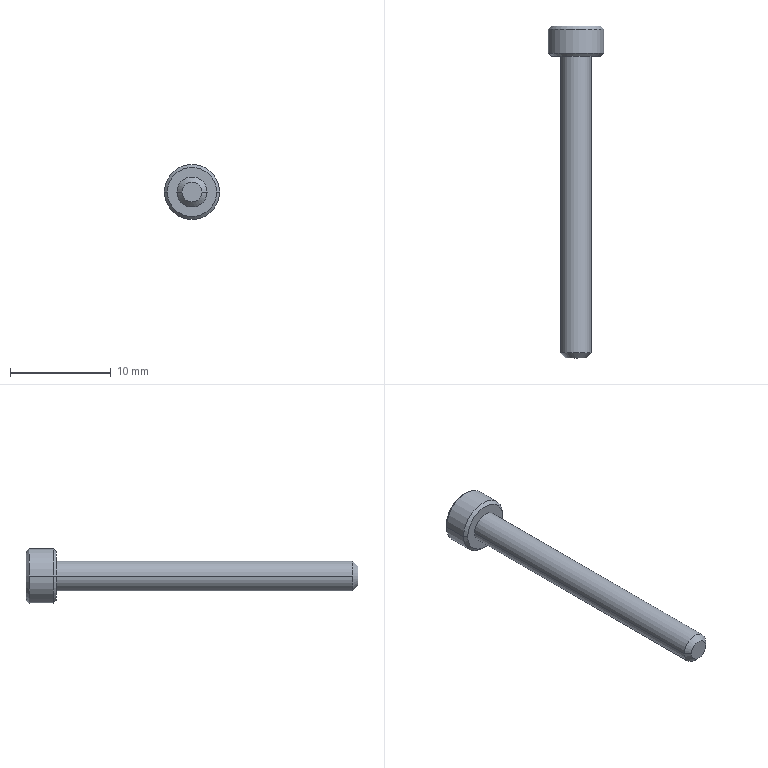Part | STEP file | BB62-M3-30L-3 | 1 solid | 27 faces | box 5.5 x 33 x 5.5 mm | volume 272.045 mm3 | plane 15 | cone 8 | cylinder 4 | commonest cylinder face diameters 3 x2 5.5 x2
STEP:
#1=CARTESIAN_POINT('',(0.,0.8715,0.));
#2=VERTEX_POINT('',#1);
#3=CARTESIAN_POINT('',(1.435,1.7,0.));
#4=VERTEX_POINT('',#3);
#5=CARTESIAN_POINT('',(0.,0.8715,0.));
#6=DIRECTION('',(0.866,0.5,0.));
#7=VECTOR('',#6,1000.);
#8=LINE('',#5,#7);
#9=EDGE_CURVE('',#2,#4,#8,.T.);
#10=ORIENTED_EDGE('',*,*,#9,.F.);
#11=CARTESIAN_POINT('',(-1.435,1.7,0.));
#12=VERTEX_POINT('',#11);
#13=CARTESIAN_POINT('',(0.,0.8715,0.));
#14=DIRECTION('',(-0.866,0.5,0.));
#15=VECTOR('',#14,1000.);
#16=LINE('',#13,#15);
#17=EDGE_CURVE('',#2,#12,#16,.T.);
#18=ORIENTED_EDGE('',*,*,#17,.T.);
#19=CARTESIAN_POINT('',(-1.243,1.7,0.7175));
#20=VERTEX_POINT('',#19);
#21=CARTESIAN_POINT('',(0.,1.7,0.));
#22=DIRECTION('',(0.,-1.,0.));
#23=DIRECTION('',(-1.,0.,0.));
#24=AXIS2_PLACEMENT_3D('',#21,#22,#23);
#25=CIRCLE('',#24,1.435);
#26=EDGE_CURVE('',#20,#12,#25,.T.);
#27=ORIENTED_EDGE('',*,*,#26,.F.);
#28=CARTESIAN_POINT('',(0.,1.7,1.435));
#29=VERTEX_POINT('',#28);
#30=CARTESIAN_POINT('',(0.,1.7,0.));
#31=DIRECTION('',(0.,-1.,0.));
#32=DIRECTION('',(-1.,0.,0.));
#33=AXIS2_PLACEMENT_3D('',#30,#31,#32);
#34=CIRCLE('',#33,1.435);
#35=EDGE_CURVE('',#29,#20,#34,.T.);
#36=ORIENTED_EDGE('',*,*,#35,.F.);
#37=CARTESIAN_POINT('',(1.243,1.7,0.7175));
#38=VERTEX_POINT('',#37);
#39=CARTESIAN_POINT('',(0.,1.7,0.));
#40=DIRECTION('',(0.,-1.,0.));
#41=DIRECTION('',(-1.,0.,0.));
#42=AXIS2_PLACEMENT_3D('',#39,#40,#41);
#43=CIRCLE('',#42,1.435);
#44=EDGE_CURVE('',#38,#29,#43,.T.);
#45=ORIENTED_EDGE('',*,*,#44,.F.);
#46=CARTESIAN_POINT('',(0.,1.7,0.));
#47=DIRECTION('',(0.,-1.,0.));
#48=DIRECTION('',(-1.,0.,0.));
#49=AXIS2_PLACEMENT_3D('',#46,#47,#48);
#50=CIRCLE('',#49,1.435);
#51=EDGE_CURVE('',#4,#38,#50,.T.);
#52=ORIENTED_EDGE('',*,*,#51,.F.);
#53=EDGE_LOOP('',(#10,#18,#27,#36,#45,#52));
#54=FACE_OUTER_BOUND('',#53,.T.);
#55=CARTESIAN_POINT('',(0.,1000.872,0.));
#56=DIRECTION('',(0.,1.,0.));
#57=DIRECTION('',(1.,0.,0.));
#58=AXIS2_PLACEMENT_3D('',#55,#56,#57);
#59=CONICAL_SURFACE('',#58,1732.051,1.047);
#60=ADVANCED_FACE('',(#54),#59,.F.);
#61=CARTESIAN_POINT('',(1.,-30.,0.));
#62=VERTEX_POINT('',#61);
#63=CARTESIAN_POINT('',(-1.,-30.,0.));
#64=VERTEX_POINT('',#63);
#65=CARTESIAN_POINT('',(0.,-30.,0.));
#66=DIRECTION('',(0.,1.,0.));
#67=DIRECTION('',(1.,0.,0.));
#68=AXIS2_PLACEMENT_3D('',#65,#66,#67);
#69=CIRCLE('',#68,1.);
#70=EDGE_CURVE('',#62,#64,#69,.T.);
#71=ORIENTED_EDGE('',*,*,#70,.T.);
#72=CARTESIAN_POINT('',(-1.5,-29.5,0.));
#73=VERTEX_POINT('',#72);
#74=CARTESIAN_POINT('',(-1.,-30.,0.));
#75=DIRECTION('',(-0.7071,0.7071,0.));
#76=VECTOR('',#75,1000.);
#77=LINE('',#74,#76);
#78=EDGE_CURVE('',#64,#73,#77,.T.);
#79=ORIENTED_EDGE('',*,*,#78,.T.);
#80=CARTESIAN_POINT('',(1.5,-29.5,0.));
#81=VERTEX_POINT('',#80);
#82=CARTESIAN_POINT('',(0.,-29.5,0.));
#83=DIRECTION('',(0.,-1.,0.));
#84=DIRECTION('',(-1.,0.,0.));
#85=AXIS2_PLACEMENT_3D('',#82,#83,#84);
#86=CIRCLE('',#85,1.5);
#87=EDGE_CURVE('',#73,#81,#86,.T.);
#88=ORIENTED_EDGE('',*,*,#87,.T.);
#89=CARTESIAN_POINT('',(1.,-30.,0.));
#90=DIRECTION('',(0.7071,0.7071,0.));
#91=VECTOR('',#90,1000.);
#92=LINE('',#89,#91);
#93=EDGE_CURVE('',#62,#81,#92,.T.);
#94=ORIENTED_EDGE('',*,*,#93,.F.);
#95=EDGE_LOOP('',(#71,#79,#88,#94));
#96=FACE_OUTER_BOUND('',#95,.T.);
#97=CARTESIAN_POINT('',(0.,-30.,0.));
#98=DIRECTION('',(0.,1.,0.));
#99=DIRECTION('',(1.,0.,0.));
#100=AXIS2_PLACEMENT_3D('',#97,#98,#99);
#101=CONICAL_SURFACE('',#100,1.,0.7854);
#102=ADVANCED_FACE('',(#96),#101,.T.);
#103=ORIENTED_EDGE('',*,*,#87,.F.);
#104=CARTESIAN_POINT('',(-1.5,0.,0.));
#105=VERTEX_POINT('',#104);
#106=CARTESIAN_POINT('',(-1.5,-29.5,0.));
#107=DIRECTION('',(0.,1.,0.));
#108=VECTOR('',#107,1000.);
#109=LINE('',#106,#108);
#110=EDGE_CURVE('',#73,#105,#109,.T.);
#111=ORIENTED_EDGE('',*,*,#110,.T.);
#112=CARTESIAN_POINT('',(1.5,0.,0.));
#113=VERTEX_POINT('',#112);
#114=CARTESIAN_POINT('',(0.,0.,0.));
#115=DIRECTION('',(0.,-1.,0.));
#116=DIRECTION('',(-1.,0.,0.));
#117=AXIS2_PLACEMENT_3D('',#114,#115,#116);
#118=CIRCLE('',#117,1.5);
#119=EDGE_CURVE('',#105,#113,#118,.T.);
#120=ORIENTED_EDGE('',*,*,#119,.T.);
#121=CARTESIAN_POINT('',(1.5,-29.5,0.));
#122=DIRECTION('',(0.,1.,0.));
#123=VECTOR('',#122,1000.);
#124=LINE('',#121,#123);
#125=EDGE_CURVE('',#81,#113,#124,.T.);
#126=ORIENTED_EDGE('',*,*,#125,.F.);
#127=EDGE_LOOP('',(#103,#111,#120,#126));
#128=FACE_OUTER_BOUND('',#127,.T.);
#129=CARTESIAN_POINT('',(0.,-29.5,0.));
#130=DIRECTION('',(0.,1.,0.));
#131=DIRECTION('',(1.,0.,0.));
#132=AXIS2_PLACEMENT_3D('',#129,#130,#131);
#133=CYLINDRICAL_SURFACE('',#132,1.5);
#134=ADVANCED_FACE('',(#128),#133,.T.);
#135=CARTESIAN_POINT('',(-2.45,3.,0.));
#136=VERTEX_POINT('',#135);
#137=CARTESIAN_POINT('',(2.45,3.,0.));
#138=VERTEX_POINT('',#137);
#139=CARTESIAN_POINT('',(0.,3.,0.));
#140=DIRECTION('',(0.,-1.,0.));
#141=DIRECTION('',(-1.,0.,0.));
#142=AXIS2_PLACEMENT_3D('',#139,#140,#141);
#143=CIRCLE('',#142,2.45);
#144=EDGE_CURVE('',#136,#138,#143,.T.);
#145=ORIENTED_EDGE('',*,*,#144,.T.);
#146=CARTESIAN_POINT('',(2.75,2.7,0.));
#147=VERTEX_POINT('',#146);
#148=CARTESIAN_POINT('',(2.75,2.7,0.));
#149=DIRECTION('',(0.7071,-0.7071,0.));
#150=VECTOR('',#149,1000.);
#151=LINE('',#148,#150);
#152=EDGE_CURVE('',#138,#147,#151,.T.);
#153=ORIENTED_EDGE('',*,*,#152,.T.);
#154=CARTESIAN_POINT('',(-2.75,2.7,0.));
#155=VERTEX_POINT('',#154);
#156=CARTESIAN_POINT('',(0.,2.7,0.));
#157=DIRECTION('',(0.,-1.,0.));
#158=DIRECTION('',(-1.,0.,0.));
#159=AXIS2_PLACEMENT_3D('',#156,#157,#158);
#160=CIRCLE('',#159,2.75);
#161=EDGE_CURVE('',#155,#147,#160,.T.);
#162=ORIENTED_EDGE('',*,*,#161,.F.);
#163=CARTESIAN_POINT('',(-2.75,2.7,0.));
#164=DIRECTION('',(-0.7071,-0.7071,0.));
#165=VECTOR('',#164,1000.);
#166=LINE('',#163,#165);
#167=EDGE_CURVE('',#136,#155,#166,.T.);
#168=ORIENTED_EDGE('',*,*,#167,.F.);
#169=EDGE_LOOP('',(#145,#153,#162,#168));
#170=FACE_OUTER_BOUND('',#169,.T.);
#171=CARTESIAN_POINT('',(0.,2.7,0.));
#172=DIRECTION('',(0.,-1.,0.));
#173=DIRECTION('',(-1.,0.,0.));
#174=AXIS2_PLACEMENT_3D('',#171,#172,#173);
#175=CONICAL_SURFACE('',#174,2.75,0.7854);
#176=ADVANCED_FACE('',(#170),#175,.T.);
#177=ORIENTED_EDGE('',*,*,#161,.T.);
#178=CARTESIAN_POINT('',(2.75,0.3,0.));
#179=VERTEX_POINT('',#178);
#180=CARTESIAN_POINT('',(2.75,1.62,0.));
#181=DIRECTION('',(0.,-1.,0.));
#182=VECTOR('',#181,1000.);
#183=LINE('',#180,#182);
#184=EDGE_CURVE('',#147,#179,#183,.T.);
#185=ORIENTED_EDGE('',*,*,#184,.T.);
#186=CARTESIAN_POINT('',(-2.75,0.3,0.));
#187=VERTEX_POINT('',#186);
#188=CARTESIAN_POINT('',(0.,0.3,0.));
#189=DIRECTION('',(0.,-1.,0.));
#190=DIRECTION('',(-1.,0.,0.));
#191=AXIS2_PLACEMENT_3D('',#188,#189,#190);
#192=CIRCLE('',#191,2.75);
#193=EDGE_CURVE('',#187,#179,#192,.T.);
#194=ORIENTED_EDGE('',*,*,#193,.F.);
#195=CARTESIAN_POINT('',(-2.75,1.62,0.));
#196=DIRECTION('',(0.,-1.,0.));
#197=VECTOR('',#196,1000.);
#198=LINE('',#195,#197);
#199=EDGE_CURVE('',#155,#187,#198,.T.);
#200=ORIENTED_EDGE('',*,*,#199,.F.);
#201=EDGE_LOOP('',(#177,#185,#194,#200));
#202=FACE_OUTER_BOUND('',#201,.T.);
#203=CARTESIAN_POINT('',(0.,1.62,0.));
#204=DIRECTION('',(0.,-1.,0.));
#205=DIRECTION('',(-1.,0.,0.));
#206=AXIS2_PLACEMENT_3D('',#203,#204,#205);
#207=CYLINDRICAL_SURFACE('',#206,2.75);
#208=ADVANCED_FACE('',(#202),#207,.T.);
#209=CARTESIAN_POINT('',(-2.45,0.,0.));
#210=VERTEX_POINT('',#209);
#211=CARTESIAN_POINT('',(2.45,0.,0.));
#212=VERTEX_POINT('',#211);
#213=CARTESIAN_POINT('',(0.,0.,0.));
#214=DIRECTION('',(0.,-1.,0.));
#215=DIRECTION('',(-1.,0.,0.));
#216=AXIS2_PLACEMENT_3D('',#213,#214,#215);
#217=CIRCLE('',#216,2.45);
#218=EDGE_CURVE('',#210,#212,#217,.T.);
#219=ORIENTED_EDGE('',*,*,#218,.F.);
#220=CARTESIAN_POINT('',(-2.45,0.,0.));
#221=DIRECTION('',(-0.7071,0.7071,0.));
#222=VECTOR('',#221,1000.);
#223=LINE('',#220,#222);
#224=EDGE_CURVE('',#210,#187,#223,.T.);
#225=ORIENTED_EDGE('',*,*,#224,.T.);
#226=ORIENTED_EDGE('',*,*,#193,.T.);
#227=CARTESIAN_POINT('',(2.45,0.,0.));
#228=DIRECTION('',(0.7071,0.7071,0.));
#229=VECTOR('',#228,1000.);
#230=LINE('',#227,#229);
#231=EDGE_CURVE('',#212,#179,#230,.T.);
#232=ORIENTED_EDGE('',*,*,#231,.F.);
#233=EDGE_LOOP('',(#219,#225,#226,#232));
#234=FACE_OUTER_BOUND('',#233,.T.);
#235=CARTESIAN_POINT('',(0.,0.,0.));
#236=DIRECTION('',(0.,1.,0.));
#237=DIRECTION('',(1.,0.,0.));
#238=AXIS2_PLACEMENT_3D('',#235,#236,#237);
#239=CONICAL_SURFACE('',#238,2.45,0.7854);
#240=ADVANCED_FACE('',(#234),#239,.T.);
#241=ORIENTED_EDGE('',*,*,#144,.F.);
#242=CARTESIAN_POINT('',(0.,3.,0.));
#243=DIRECTION('',(0.,-1.,0.));
#244=DIRECTION('',(-1.,0.,0.));
#245=AXIS2_PLACEMENT_3D('',#242,#243,#244);
#246=CIRCLE('',#245,2.45);
#247=EDGE_CURVE('',#138,#136,#246,.T.);
#248=ORIENTED_EDGE('',*,*,#247,.F.);
#249=EDGE_LOOP('',(#241,#248));
#250=FACE_OUTER_BOUND('',#249,.T.);
#251=CARTESIAN_POINT('',(0.,3.,-1.435));
#252=VERTEX_POINT('',#251);
#253=CARTESIAN_POINT('',(-1.243,3.,-0.7175));
#254=VERTEX_POINT('',#253);
#255=CARTESIAN_POINT('',(0.,3.,-1.435));
#256=DIRECTION('',(-0.866,0.,0.5));
#257=VECTOR('',#256,1000.);
#258=LINE('',#255,#257);
#259=EDGE_CURVE('',#252,#254,#258,.T.);
#260=ORIENTED_EDGE('',*,*,#259,.F.);
#261=CARTESIAN_POINT('',(1.243,3.,-0.7175));
#262=VERTEX_POINT('',#261);
#263=CARTESIAN_POINT('',(1.243,3.,-0.7175));
#264=DIRECTION('',(-0.866,0.,-0.5));
#265=VECTOR('',#264,1000.);
#266=LINE('',#263,#265);
#267=EDGE_CURVE('',#262,#252,#266,.T.);
#268=ORIENTED_EDGE('',*,*,#267,.F.);
#269=CARTESIAN_POINT('',(1.243,3.,0.7175));
#270=VERTEX_POINT('',#269);
#271=CARTESIAN_POINT('',(1.243,3.,0.7175));
#272=DIRECTION('',(0.,0.,-1.));
#273=VECTOR('',#272,1000.);
#274=LINE('',#271,#273);
#275=EDGE_CURVE('',#270,#262,#274,.T.);
#276=ORIENTED_EDGE('',*,*,#275,.F.);
#277=CARTESIAN_POINT('',(0.,3.,1.435));
#278=VERTEX_POINT('',#277);
#279=CARTESIAN_POINT('',(0.,3.,1.435));
#280=DIRECTION('',(0.866,0.,-0.5));
#281=VECTOR('',#280,1000.);
#282=LINE('',#279,#281);
#283=EDGE_CURVE('',#278,#270,#282,.T.);
#284=ORIENTED_EDGE('',*,*,#283,.F.);
#285=CARTESIAN_POINT('',(-1.243,3.,0.7175));
#286=VERTEX_POINT('',#285);
#287=CARTESIAN_POINT('',(-1.243,3.,0.7175));
#288=DIRECTION('',(0.866,0.,0.5));
#289=VECTOR('',#288,1000.);
#290=LINE('',#287,#289);
#291=EDGE_CURVE('',#286,#278,#290,.T.);
#292=ORIENTED_EDGE('',*,*,#291,.F.);
#293=CARTESIAN_POINT('',(-1.243,3.,-0.7175));
#294=DIRECTION('',(0.,0.,1.));
#295=VECTOR('',#294,1000.);
#296=LINE('',#293,#295);
#297=EDGE_CURVE('',#254,#286,#296,.T.);
#298=ORIENTED_EDGE('',*,*,#297,.F.);
#299=EDGE_LOOP('',(#260,#268,#276,#284,#292,#298));
#300=FACE_BOUND('',#299,.T.);
#301=CARTESIAN_POINT('',(2.45,3.,0.));
#302=DIRECTION('',(0.,1.,0.));
#303=DIRECTION('',(1.,0.,0.));
#304=AXIS2_PLACEMENT_3D('',#301,#302,#303);
#305=PLANE('',#304);
#306=ADVANCED_FACE('',(#250,#300),#305,.T.);
#307=CARTESIAN_POINT('',(0.,0.,0.));
#308=DIRECTION('',(0.,-1.,0.));
#309=DIRECTION('',(-1.,0.,0.));
#310=AXIS2_PLACEMENT_3D('',#307,#308,#309);
#311=CIRCLE('',#310,1.5);
#312=EDGE_CURVE('',#113,#105,#311,.T.);
#313=ORIENTED_EDGE('',*,*,#312,.F.);
#314=ORIENTED_EDGE('',*,*,#119,.F.);
#315=EDGE_LOOP('',(#313,#314));
#316=FACE_BOUND('',#315,.T.);
#317=CARTESIAN_POINT('',(0.,0.,0.));
#318=DIRECTION('',(0.,-1.,0.));
#319=DIRECTION('',(-1.,0.,0.));
#320=AXIS2_PLACEMENT_3D('',#317,#318,#319);
#321=CIRCLE('',#320,2.45);
#322=EDGE_CURVE('',#212,#210,#321,.T.);
#323=ORIENTED_EDGE('',*,*,#322,.T.);
#324=ORIENTED_EDGE('',*,*,#218,.T.);
#325=EDGE_LOOP('',(#323,#324));
#326=FACE_OUTER_BOUND('',#325,.T.);
#327=CARTESIAN_POINT('',(0.,0.,0.));
#328=DIRECTION('',(0.,-1.,0.));
#329=DIRECTION('',(-1.,0.,0.));
#330=AXIS2_PLACEMENT_3D('',#327,#328,#329);
#331=PLANE('',#330);
#332=ADVANCED_FACE('',(#316,#326),#331,.T.);
#333=ORIENTED_EDGE('',*,*,#224,.F.);
#334=ORIENTED_EDGE('',*,*,#322,.F.);
#335=ORIENTED_EDGE('',*,*,#231,.T.);
#336=CARTESIAN_POINT('',(0.,0.3,0.));
#337=DIRECTION('',(0.,-1.,0.));
#338=DIRECTION('',(-1.,0.,0.));
#339=AXIS2_PLACEMENT_3D('',#336,#337,#338);
#340=CIRCLE('',#339,2.75);
#341=EDGE_CURVE('',#179,#187,#340,.T.);
#342=ORIENTED_EDGE('',*,*,#341,.T.);
#343=EDGE_LOOP('',(#333,#334,#335,#342));
#344=FACE_OUTER_BOUND('',#343,.T.);
#345=CARTESIAN_POINT('',(0.,0.,0.));
#346=DIRECTION('',(0.,1.,0.));
#347=DIRECTION('',(1.,0.,0.));
#348=AXIS2_PLACEMENT_3D('',#345,#346,#347);
#349=CONICAL_SURFACE('',#348,2.45,0.7854);
#350=ADVANCED_FACE('',(#344),#349,.T.);
#351=ORIENTED_EDGE('',*,*,#184,.F.);
#352=CARTESIAN_POINT('',(0.,2.7,0.));
#353=DIRECTION('',(0.,-1.,0.));
#354=DIRECTION('',(-1.,0.,0.));
#355=AXIS2_PLACEMENT_3D('',#352,#353,#354);
#356=CIRCLE('',#355,2.75);
#357=EDGE_CURVE('',#147,#155,#356,.T.);
#358=ORIENTED_EDGE('',*,*,#357,.T.);
#359=ORIENTED_EDGE('',*,*,#199,.T.);
#360=ORIENTED_EDGE('',*,*,#341,.F.);
#361=EDGE_LOOP('',(#351,#358,#359,#360));
#362=FACE_OUTER_BOUND('',#361,.T.);
#363=CARTESIAN_POINT('',(0.,1.62,0.));
#364=DIRECTION('',(0.,-1.,0.));
#365=DIRECTION('',(-1.,0.,0.));
#366=AXIS2_PLACEMENT_3D('',#363,#364,#365);
#367=CYLINDRICAL_SURFACE('',#366,2.75);
#368=ADVANCED_FACE('',(#362),#367,.T.);
#369=ORIENTED_EDGE('',*,*,#152,.F.);
#370=ORIENTED_EDGE('',*,*,#247,.T.);
#371=ORIENTED_EDGE('',*,*,#167,.T.);
#372=ORIENTED_EDGE('',*,*,#357,.F.);
#373=EDGE_LOOP('',(#369,#370,#371,#372));
#374=FACE_OUTER_BOUND('',#373,.T.);
#375=CARTESIAN_POINT('',(0.,2.7,0.));
#376=DIRECTION('',(0.,-1.,0.));
#377=DIRECTION('',(-1.,0.,0.));
#378=AXIS2_PLACEMENT_3D('',#375,#376,#377);
#379=CONICAL_SURFACE('',#378,2.75,0.7854);
#380=ADVANCED_FACE('',(#374),#379,.T.);
#381=ORIENTED_EDGE('',*,*,#110,.F.);
#382=CARTESIAN_POINT('',(0.,-29.5,0.));
#383=DIRECTION('',(0.,-1.,0.));
#384=DIRECTION('',(-1.,0.,0.));
#385=AXIS2_PLACEMENT_3D('',#382,#383,#384);
#386=CIRCLE('',#385,1.5);
#387=EDGE_CURVE('',#81,#73,#386,.T.);
#388=ORIENTED_EDGE('',*,*,#387,.F.);
#389=ORIENTED_EDGE('',*,*,#125,.T.);
#390=ORIENTED_EDGE('',*,*,#312,.T.);
#391=EDGE_LOOP('',(#381,#388,#389,#390));
#392=FACE_OUTER_BOUND('',#391,.T.);
#393=CARTESIAN_POINT('',(0.,-29.5,0.));
#394=DIRECTION('',(0.,1.,0.));
#395=DIRECTION('',(1.,0.,0.));
#396=AXIS2_PLACEMENT_3D('',#393,#394,#395);
#397=CYLINDRICAL_SURFACE('',#396,1.5);
#398=ADVANCED_FACE('',(#392),#397,.T.);
#399=ORIENTED_EDGE('',*,*,#70,.F.);
#400=CARTESIAN_POINT('',(0.,-30.,0.));
#401=DIRECTION('',(0.,1.,0.));
#402=DIRECTION('',(1.,0.,0.));
#403=AXIS2_PLACEMENT_3D('',#400,#401,#402);
#404=CIRCLE('',#403,1.);
#405=EDGE_CURVE('',#64,#62,#404,.T.);
#406=ORIENTED_EDGE('',*,*,#405,.F.);
#407=EDGE_LOOP('',(#399,#406));
#408=FACE_OUTER_BOUND('',#407,.T.);
#409=CARTESIAN_POINT('',(0.,-30.,0.));
#410=DIRECTION('',(0.,-1.,0.));
#411=DIRECTION('',(-1.,0.,0.));
#412=AXIS2_PLACEMENT_3D('',#409,#410,#411);
#413=PLANE('',#412);
#414=ADVANCED_FACE('',(#408),#413,.T.);
#415=ORIENTED_EDGE('',*,*,#78,.F.);
#416=ORIENTED_EDGE('',*,*,#405,.T.);
#417=ORIENTED_EDGE('',*,*,#93,.T.);
#418=ORIENTED_EDGE('',*,*,#387,.T.);
#419=EDGE_LOOP('',(#415,#416,#417,#418));
#420=FACE_OUTER_BOUND('',#419,.T.);
#421=CARTESIAN_POINT('',(0.,-30.,0.));
#422=DIRECTION('',(0.,1.,0.));
#423=DIRECTION('',(1.,0.,0.));
#424=AXIS2_PLACEMENT_3D('',#421,#422,#423);
#425=CONICAL_SURFACE('',#424,1.,0.7854);
#426=ADVANCED_FACE('',(#420),#425,.T.);
#427=CARTESIAN_POINT('',(1.243,1.7,-0.7175));
#428=VERTEX_POINT('',#427);
#429=CARTESIAN_POINT('',(0.,1.7,-1.435));
#430=VERTEX_POINT('',#429);
#431=CARTESIAN_POINT('',(1.243,1.7,-0.7175));
#432=DIRECTION('',(-0.866,0.,-0.5));
#433=VECTOR('',#432,1000.);
#434=LINE('',#431,#433);
#435=EDGE_CURVE('',#428,#430,#434,.T.);
#436=ORIENTED_EDGE('',*,*,#435,.F.);
#437=CARTESIAN_POINT('',(1.243,3.,-0.7175));
#438=DIRECTION('',(0.,-1.,0.));
#439=VECTOR('',#438,1000.);
#440=LINE('',#437,#439);
#441=EDGE_CURVE('',#262,#428,#440,.T.);
#442=ORIENTED_EDGE('',*,*,#441,.F.);
#443=ORIENTED_EDGE('',*,*,#267,.T.);
#444=CARTESIAN_POINT('',(0.,3.,-1.435));
#445=DIRECTION('',(0.,-1.,0.));
#446=VECTOR('',#445,1000.);
#447=LINE('',#444,#446);
#448=EDGE_CURVE('',#252,#430,#447,.T.);
#449=ORIENTED_EDGE('',*,*,#448,.T.);
#450=EDGE_LOOP('',(#436,#442,#443,#449));
#451=FACE_OUTER_BOUND('',#450,.T.);
#452=CARTESIAN_POINT('',(1.243,3.,-0.7175));
#453=DIRECTION('',(-0.5,0.,0.866));
#454=DIRECTION('',(0.866,0.,0.5));
#455=AXIS2_PLACEMENT_3D('',#452,#453,#454);
#456=PLANE('',#455);
#457=ADVANCED_FACE('',(#451),#456,.T.);
#458=CARTESIAN_POINT('',(-1.243,1.7,-0.7175));
#459=VERTEX_POINT('',#458);
#460=CARTESIAN_POINT('',(0.,1.7,-1.435));
#461=DIRECTION('',(-0.866,0.,0.5));
#462=VECTOR('',#461,1000.);
#463=LINE('',#460,#462);
#464=EDGE_CURVE('',#430,#459,#463,.T.);
#465=ORIENTED_EDGE('',*,*,#464,.F.);
#466=ORIENTED_EDGE('',*,*,#448,.F.);
#467=ORIENTED_EDGE('',*,*,#259,.T.);
#468=CARTESIAN_POINT('',(-1.243,3.,-0.7175));
#469=DIRECTION('',(0.,-1.,0.));
#470=VECTOR('',#469,1000.);
#471=LINE('',#468,#470);
#472=EDGE_CURVE('',#254,#459,#471,.T.);
#473=ORIENTED_EDGE('',*,*,#472,.T.);
#474=EDGE_LOOP('',(#465,#466,#467,#473));
#475=FACE_OUTER_BOUND('',#474,.T.);
#476=CARTESIAN_POINT('',(0.,3.,-1.435));
#477=DIRECTION('',(0.5,0.,0.866));
#478=DIRECTION('',(0.866,0.,-0.5));
#479=AXIS2_PLACEMENT_3D('',#476,#477,#478);
#480=PLANE('',#479);
#481=ADVANCED_FACE('',(#475),#480,.T.);
#482=CARTESIAN_POINT('',(-1.243,1.7,-0.7175));
#483=DIRECTION('',(0.,0.,1.));
#484=VECTOR('',#483,1000.);
#485=LINE('',#482,#484);
#486=EDGE_CURVE('',#459,#20,#485,.T.);
#487=ORIENTED_EDGE('',*,*,#486,.F.);
#488=ORIENTED_EDGE('',*,*,#472,.F.);
#489=ORIENTED_EDGE('',*,*,#297,.T.);
#490=CARTESIAN_POINT('',(-1.243,3.,0.7175));
#491=DIRECTION('',(0.,-1.,0.));
#492=VECTOR('',#491,1000.);
#493=LINE('',#490,#492);
#494=EDGE_CURVE('',#286,#20,#493,.T.);
#495=ORIENTED_EDGE('',*,*,#494,.T.);
#496=EDGE_LOOP('',(#487,#488,#489,#495));
#497=FACE_OUTER_BOUND('',#496,.T.);
#498=CARTESIAN_POINT('',(-1.243,3.,-0.7175));
#499=DIRECTION('',(1.,0.,0.));
#500=DIRECTION('',(0.,0.,-1.));
#501=AXIS2_PLACEMENT_3D('',#498,#499,#500);
#502=PLANE('',#501);
#503=ADVANCED_FACE('',(#497),#502,.T.);
#504=CARTESIAN_POINT('',(-1.243,1.7,0.7175));
#505=DIRECTION('',(0.866,0.,0.5));
#506=VECTOR('',#505,1000.);
#507=LINE('',#504,#506);
#508=EDGE_CURVE('',#20,#29,#507,.T.);
#509=ORIENTED_EDGE('',*,*,#508,.F.);
#510=ORIENTED_EDGE('',*,*,#494,.F.);
#511=ORIENTED_EDGE('',*,*,#291,.T.);
#512=CARTESIAN_POINT('',(0.,3.,1.435));
#513=DIRECTION('',(0.,-1.,0.));
#514=VECTOR('',#513,1000.);
#515=LINE('',#512,#514);
#516=EDGE_CURVE('',#278,#29,#515,.T.);
#517=ORIENTED_EDGE('',*,*,#516,.T.);
#518=EDGE_LOOP('',(#509,#510,#511,#517));
#519=FACE_OUTER_BOUND('',#518,.T.);
#520=CARTESIAN_POINT('',(-1.243,3.,0.7175));
#521=DIRECTION('',(0.5,0.,-0.866));
#522=DIRECTION('',(-0.866,0.,-0.5));
#523=AXIS2_PLACEMENT_3D('',#520,#521,#522);
#524=PLANE('',#523);
#525=ADVANCED_FACE('',(#519),#524,.T.);
#526=CARTESIAN_POINT('',(0.,1.7,1.435));
#527=DIRECTION('',(0.866,0.,-0.5));
#528=VECTOR('',#527,1000.);
#529=LINE('',#526,#528);
#530=EDGE_CURVE('',#29,#38,#529,.T.);
#531=ORIENTED_EDGE('',*,*,#530,.F.);
#532=ORIENTED_EDGE('',*,*,#516,.F.);
#533=ORIENTED_EDGE('',*,*,#283,.T.);
#534=CARTESIAN_POINT('',(1.243,3.,0.7175));
#535=DIRECTION('',(0.,-1.,0.));
#536=VECTOR('',#535,1000.);
#537=LINE('',#534,#536);
#538=EDGE_CURVE('',#270,#38,#537,.T.);
#539=ORIENTED_EDGE('',*,*,#538,.T.);
#540=EDGE_LOOP('',(#531,#532,#533,#539));
#541=FACE_OUTER_BOUND('',#540,.T.);
#542=CARTESIAN_POINT('',(0.,3.,1.435));
#543=DIRECTION('',(-0.5,0.,-0.866));
#544=DIRECTION('',(-0.866,0.,0.5));
#545=AXIS2_PLACEMENT_3D('',#542,#543,#544);
#546=PLANE('',#545);
#547=ADVANCED_FACE('',(#541),#546,.T.);
#548=CARTESIAN_POINT('',(1.243,1.7,0.7175));
#549=DIRECTION('',(0.,0.,-1.));
#550=VECTOR('',#549,1000.);
#551=LINE('',#548,#550);
#552=EDGE_CURVE('',#38,#428,#551,.T.);
#553=ORIENTED_EDGE('',*,*,#552,.F.);
#554=ORIENTED_EDGE('',*,*,#538,.F.);
#555=ORIENTED_EDGE('',*,*,#275,.T.);
#556=ORIENTED_EDGE('',*,*,#441,.T.);
#557=EDGE_LOOP('',(#553,#554,#555,#556));
#558=FACE_OUTER_BOUND('',#557,.T.);
#559=CARTESIAN_POINT('',(1.243,3.,0.7175));
#560=DIRECTION('',(-1.,0.,0.));
#561=DIRECTION('',(0.,0.,1.));
#562=AXIS2_PLACEMENT_3D('',#559,#560,#561);
#563=PLANE('',#562);
#564=ADVANCED_FACE('',(#558),#563,.T.);
#565=ORIENTED_EDGE('',*,*,#435,.T.);
#566=CARTESIAN_POINT('',(0.,1.7,0.));
#567=DIRECTION('',(0.,-1.,0.));
#568=DIRECTION('',(-1.,0.,0.));
#569=AXIS2_PLACEMENT_3D('',#566,#567,#568);
#570=CIRCLE('',#569,1.435);
#571=EDGE_CURVE('',#430,#428,#570,.T.);
#572=ORIENTED_EDGE('',*,*,#571,.T.);
#573=EDGE_LOOP('',(#565,#572));
#574=FACE_OUTER_BOUND('',#573,.T.);
#575=CARTESIAN_POINT('',(0.,1.7,0.));
#576=DIRECTION('',(0.,1.,0.));
#577=DIRECTION('',(1.,0.,0.));
#578=AXIS2_PLACEMENT_3D('',#575,#576,#577);
#579=PLANE('',#578);
#580=ADVANCED_FACE('',(#574),#579,.F.);
#581=ORIENTED_EDGE('',*,*,#552,.T.);
#582=CARTESIAN_POINT('',(0.,1.7,0.));
#583=DIRECTION('',(0.,-1.,0.));
#584=DIRECTION('',(-1.,0.,0.));
#585=AXIS2_PLACEMENT_3D('',#582,#583,#584);
#586=CIRCLE('',#585,1.435);
#587=EDGE_CURVE('',#428,#4,#586,.T.);
#588=ORIENTED_EDGE('',*,*,#587,.T.);
#589=ORIENTED_EDGE('',*,*,#51,.T.);
#590=EDGE_LOOP('',(#581,#588,#589));
#591=FACE_OUTER_BOUND('',#590,.T.);
#592=CARTESIAN_POINT('',(0.,1.7,0.));
#593=DIRECTION('',(0.,1.,0.));
#594=DIRECTION('',(1.,0.,0.));
#595=AXIS2_PLACEMENT_3D('',#592,#593,#594);
#596=PLANE('',#595);
#597=ADVANCED_FACE('',(#591),#596,.F.);
#598=ORIENTED_EDGE('',*,*,#530,.T.);
#599=ORIENTED_EDGE('',*,*,#44,.T.);
#600=EDGE_LOOP('',(#598,#599));
#601=FACE_OUTER_BOUND('',#600,.T.);
#602=CARTESIAN_POINT('',(0.,1.7,0.));
#603=DIRECTION('',(0.,1.,0.));
#604=DIRECTION('',(1.,0.,0.));
#605=AXIS2_PLACEMENT_3D('',#602,#603,#604);
#606=PLANE('',#605);
#607=ADVANCED_FACE('',(#601),#606,.F.);
#608=ORIENTED_EDGE('',*,*,#508,.T.);
#609=ORIENTED_EDGE('',*,*,#35,.T.);
#610=EDGE_LOOP('',(#608,#609));
#611=FACE_OUTER_BOUND('',#610,.T.);
#612=CARTESIAN_POINT('',(0.,1.7,0.));
#613=DIRECTION('',(0.,1.,0.));
#614=DIRECTION('',(1.,0.,0.));
#615=AXIS2_PLACEMENT_3D('',#612,#613,#614);
#616=PLANE('',#615);
#617=ADVANCED_FACE('',(#611),#616,.F.);
#618=ORIENTED_EDGE('',*,*,#486,.T.);
#619=ORIENTED_EDGE('',*,*,#26,.T.);
#620=CARTESIAN_POINT('',(0.,1.7,0.));
#621=DIRECTION('',(0.,-1.,0.));
#622=DIRECTION('',(-1.,0.,0.));
#623=AXIS2_PLACEMENT_3D('',#620,#621,#622);
#624=CIRCLE('',#623,1.435);
#625=EDGE_CURVE('',#12,#459,#624,.T.);
#626=ORIENTED_EDGE('',*,*,#625,.T.);
#627=EDGE_LOOP('',(#618,#619,#626));
#628=FACE_OUTER_BOUND('',#627,.T.);
#629=CARTESIAN_POINT('',(0.,1.7,0.));
#630=DIRECTION('',(0.,1.,0.));
#631=DIRECTION('',(1.,0.,0.));
#632=AXIS2_PLACEMENT_3D('',#629,#630,#631);
#633=PLANE('',#632);
#634=ADVANCED_FACE('',(#628),#633,.F.);
#635=ORIENTED_EDGE('',*,*,#464,.T.);
#636=CARTESIAN_POINT('',(0.,1.7,0.));
#637=DIRECTION('',(0.,-1.,0.));
#638=DIRECTION('',(-1.,0.,0.));
#639=AXIS2_PLACEMENT_3D('',#636,#637,#638);
#640=CIRCLE('',#639,1.435);
#641=EDGE_CURVE('',#459,#430,#640,.T.);
#642=ORIENTED_EDGE('',*,*,#641,.T.);
#643=EDGE_LOOP('',(#635,#642));
#644=FACE_OUTER_BOUND('',#643,.T.);
#645=CARTESIAN_POINT('',(0.,1.7,0.));
#646=DIRECTION('',(0.,1.,0.));
#647=DIRECTION('',(1.,0.,0.));
#648=AXIS2_PLACEMENT_3D('',#645,#646,#647);
#649=PLANE('',#648);
#650=ADVANCED_FACE('',(#644),#649,.F.);
#651=ORIENTED_EDGE('',*,*,#17,.F.);
#652=ORIENTED_EDGE('',*,*,#9,.T.);
#653=ORIENTED_EDGE('',*,*,#587,.F.);
#654=ORIENTED_EDGE('',*,*,#571,.F.);
#655=ORIENTED_EDGE('',*,*,#641,.F.);
#656=ORIENTED_EDGE('',*,*,#625,.F.);
#657=EDGE_LOOP('',(#651,#652,#653,#654,#655,#656));
#658=FACE_OUTER_BOUND('',#657,.T.);
#659=CARTESIAN_POINT('',(0.,1000.872,0.));
#660=DIRECTION('',(0.,1.,0.));
#661=DIRECTION('',(1.,0.,0.));
#662=AXIS2_PLACEMENT_3D('',#659,#660,#661);
#663=CONICAL_SURFACE('',#662,1732.051,1.047);
#664=ADVANCED_FACE('',(#658),#663,.F.);
#665=CLOSED_SHELL('',(#60,#102,#134,#176,#208,#240,#306,#332,#350,#368,#380,#398,#414,#426,#457,#481,#503,#525,#547,#564,#580,#597,#607,#617,#634,#650,#664));
#666=MANIFOLD_SOLID_BREP('',#665);
#667=CARTESIAN_POINT('',(0.,0.,0.));
#668=DIRECTION('',(0.,0.,1.));
#669=DIRECTION('',(1.,0.,0.));
#670=AXIS2_PLACEMENT_3D('',#667,#668,#669);
#671=(LENGTH_UNIT()NAMED_UNIT(*)SI_UNIT(.MILLI.,.METRE.));
#672=UNCERTAINTY_MEASURE_WITH_UNIT(LENGTH_MEASURE(0.00001),#671,'','');
#673=(NAMED_UNIT(*)PLANE_ANGLE_UNIT()SI_UNIT($,.RADIAN.));
#674=(NAMED_UNIT(*)SI_UNIT($,.STERADIAN.)SOLID_ANGLE_UNIT());
#675=(GEOMETRIC_REPRESENTATION_CONTEXT(3)GLOBAL_UNCERTAINTY_ASSIGNED_CONTEXT((#672))GLOBAL_UNIT_ASSIGNED_CONTEXT((#671,#673,#674))REPRESENTATION_CONTEXT('',''));
#676=ADVANCED_BREP_SHAPE_REPRESENTATION('',(#666,#670),#675);